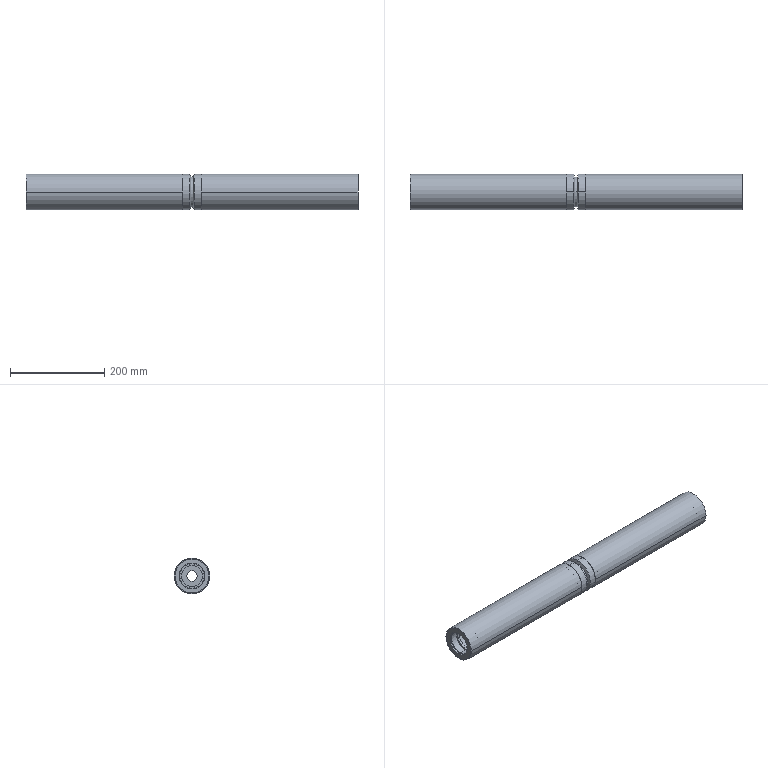Part | SolidWorks | features ICE 3, RevCut 2, Revolution 2, MirrorPattern 1 | 5 solids | 62 faces | box 705 x 76 x 76 mm | volume 640493 mm3 | cylinder 40 | plane 18 | cone 4 | commonest cylinder face diameters 72 x12 52 x8 76 x8 45 x4 55 x4 22 x2